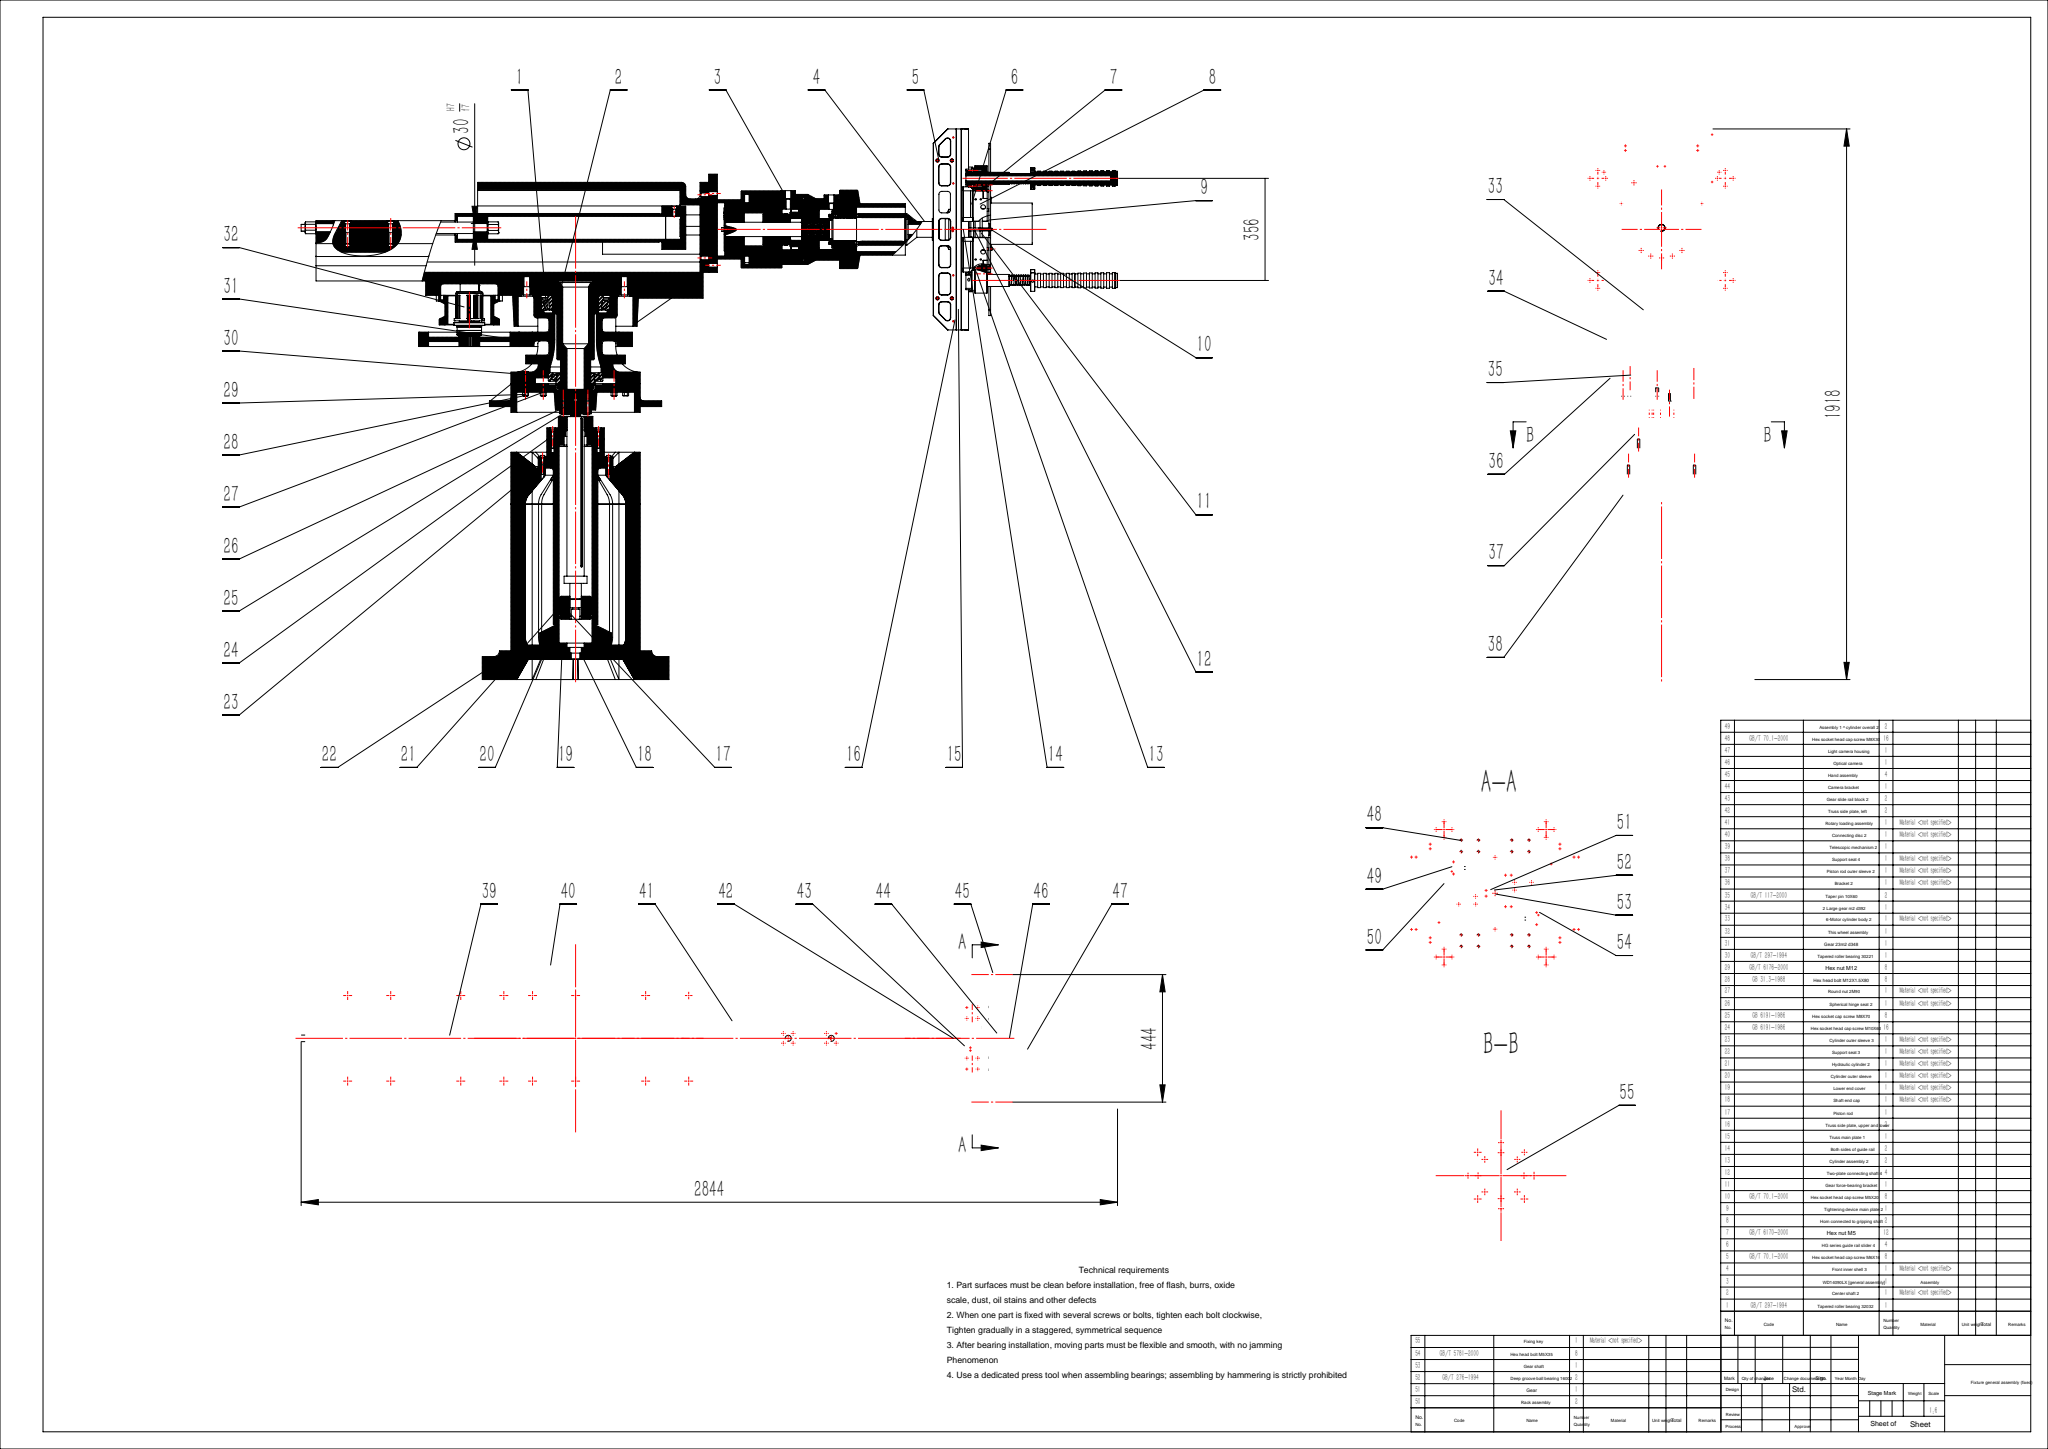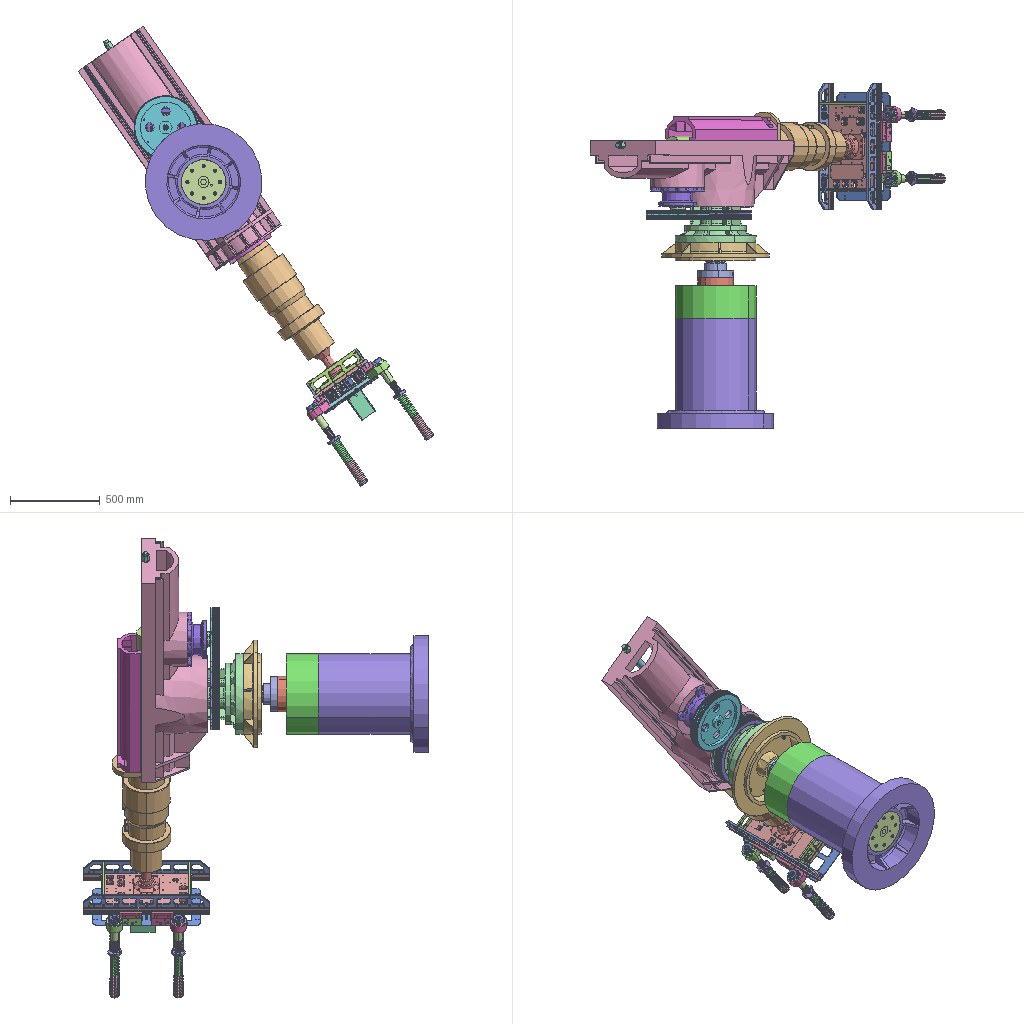Assembly | SolidWorks | 123 different items | 407 placed | box 1975 x 1918 x 2559 mm
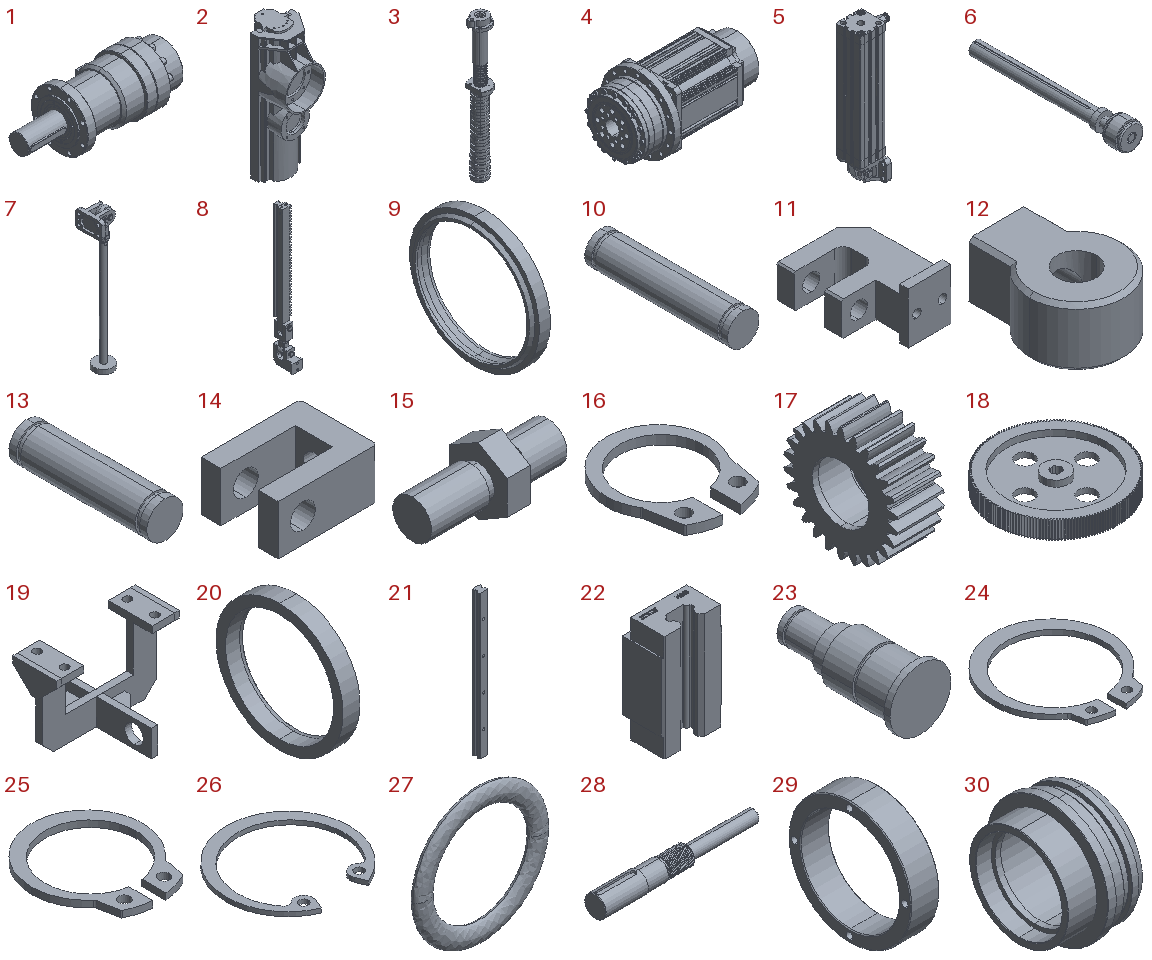Parts list (item | name | quantity | parent item | size | volume | features):
1 | (subassembly) | x1 | - | - | 15807890 mm3 | features InContextFeatHolder 12, ReferencePattern 9, CompositeCurve 5, HoleSeries 3, AEMSimFeature 1, Cut 1, LocalCirPattern 1
2 | (subassembly) | x1 | - | 440 x 501.037 x 1420 mm | 76024148 mm3 | -
3 | (subassembly) | x4 | - | 78.987 x 76 x 528 mm | 773496 mm3 | features CompositeCurve 5
4 | (subassembly) | x1 | - | 182 x 107 x 107 mm | 904156 mm3 | -
5 | (subassembly) | x2 | - | 74.5 x 58 x 297.75 mm | 433626 mm3 | -
6 | (subassembly) | x1 | - | 115 x 705.59 x 115 mm | 2459406 mm3 | -
7 | (subassembly) | x2 | - | 52 x 56 x 300.673 mm | 74670 mm3 | features CompositeCurve 1
8 | (subassembly) | x2 | - | 30 x 59.858 x 379 mm | 198364 mm3 | -
9 | - | x2 | in 1 | 6.5 x 58 x 58 mm | 3242 mm3 | features Revolution 2
10 | - | x2 | in 8 | 10 x 45 x 10 mm | 3498 mm3 | features Revolution 1
11 | - | x2 | in 8 | 45 x 57 x 30 mm | 31506 mm3 | features ICE 4, HoleWzd 3, Chamfer 2, Extrusion 1, Fillet 1
12 | - | x2 | in 8 | 24 x 32 x 15 mm | 6636 mm3 | features HoleWzd 2, Chamfer 1, Extrusion 1
13 | - | x2 | in 8 | 10 x 38 x 10 mm | 2949 mm3 | features Revolution 1
14 | - | x2 | in 8 | 40 x 31 x 20 mm | 13956 mm3 | features HoleWzd 3, Chamfer 1, Extrusion 1, ICE 1
15 | - | x2 | in 8 | 35 x 15 x 17.321 mm | 3350 mm3 | features Revolution 2, Extrusion 1
16 | - | x4 | in 8 | 11.5 x 13.997 x 1 mm | 50.603 mm3 | features Extrusion 1
17 | - | x1 | - | 23 x 55.72 x 56 mm | 29460 mm3 | features ICE 26, RevCut 1, Revolution 1
18 | - | x1 | - | 351.968 x 352 x 50 mm | 2206869 mm3 | features ICE 5, CirPattern 1, MirrorPattern 1, RefAxis 1, RevCut 1, Revolution 1
19 | - | x1 | - | 111 x 106 x 71 mm | 53566 mm3 | features BaseBody 7
20 | - | x4 | in 1 | 8 x 60 x 60 mm | 5343 mm3 | features Revolution 2
21 | - | x2 | in 8 | 15 x 15 x 270 mm | 50125 mm3 | features Draft 2, Fillet 2, ICE 2, Chamfer 1, Extrusion 1, HoleWzd 1
22 | - | x2 | - | 34 x 23.7 x 61.7 mm | 37116 mm3 | features Chamfer 35, ICE 15, Draft 12, Fillet 3, Extrusion 1, HoleWzd 1
23 | - | x1 | - | 30 x 63 x 30 mm | 23893 mm3 | features Revolution 1
24 | - | x1 | - | 28.2 x 30.881 x 1.2 mm | 270.422 mm3 | features Extrusion 1
25 | - | x1 | - | 16.8 x 19.352 x 1 mm | 87.473 mm3 | features Extrusion 1
26 | - | x1 | - | 34.4 x 33.091 x 1.2 mm | 290.13 mm3 | features Extrusion 1
27 | - | x2 | in 1 | 29.8 x 2.4 x 29.8 mm | 636.708 mm3 | features Revolution 2
28 | - | x1 | in 1 | 630 x 85 x 85 mm | 2283899 mm3 | features ICE 6, Chamfer 4, Fillet 2, CirPattern 1, Extrusion 1, Helix 1, HoleWzd 1, MirrorPattern 1, SweepCut 1
29 | - | x1 | in 1 | 35 x 150 x 150 mm | 215991 mm3 | features Chamfer 1, Extrusion 1, HoleWzd 1
30 | - | x1 | in 1 | 86 x 147 x 147 mm | 431094 mm3 | features ICE 5, Chamfer 3, Cavity 1, Extrusion 1
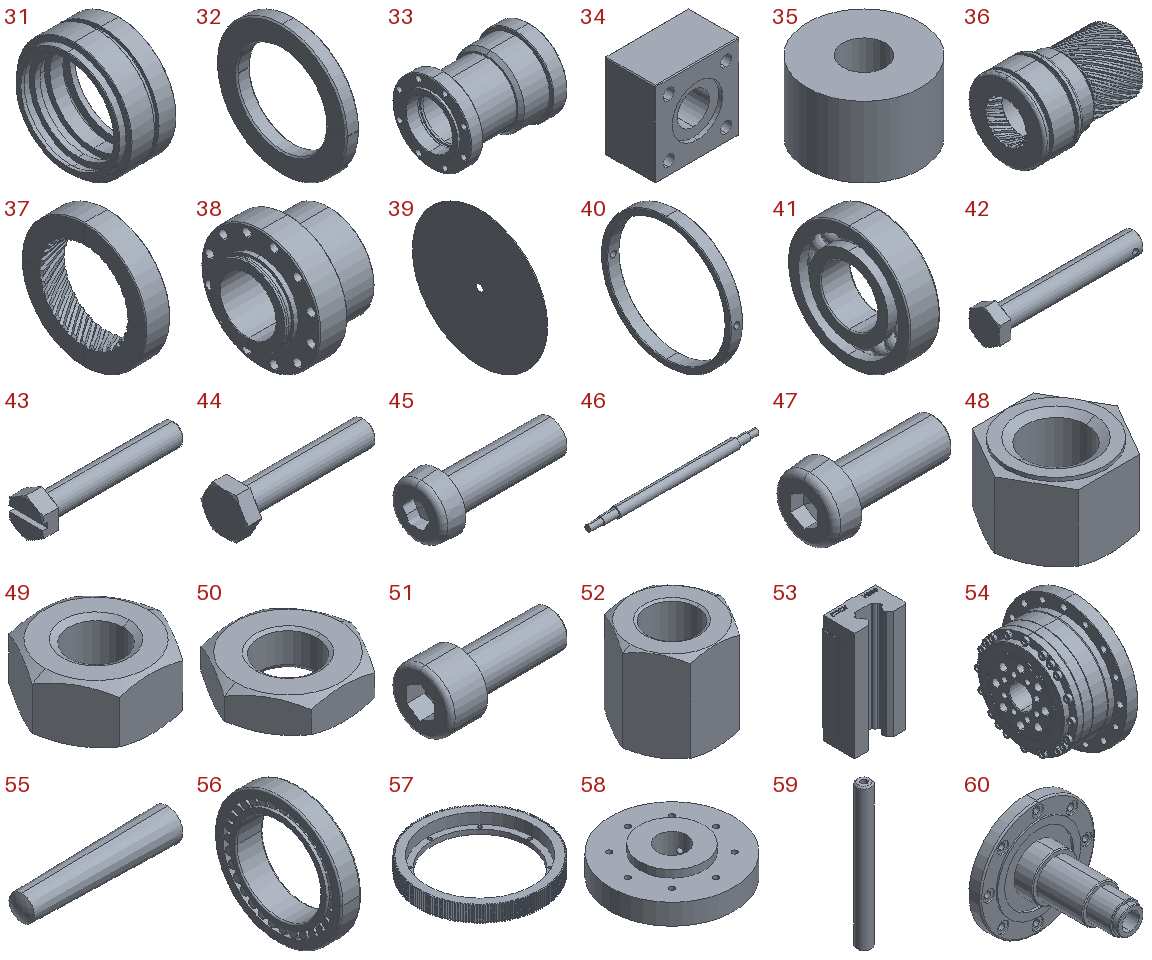31 | - | x1 | in 1 | 47 x 105 x 105 mm | 121428 mm3 | features Cavity 1, Chamfer 1, Extrusion 1, ICE 1
32 | - | x1 | in 1 | 10 x 94.999 x 95 mm | 37048 mm3 | features Chamfer 1, Extrusion 1, ICE 1
33 | - | x1 | in 1 | 317 x 249 x 249 mm | 6036986 mm3 | features Chamfer 8, HoleWzd 6, ICE 5, Cut 1, Fillet 1, LibraryFeature 1, Revolution 1
34 | - | x2 | in 1 | 50 x 30 x 50 mm | 59677 mm3 | features HoleWzd 2, Chamfer 1, Extrusion 1, ICE 1
35 | - | x1 | in 2 | 80 x 80 x 50 mm | 215984 mm3 | features Extrusion 1
36 | - | x1 | in 1 | 196 x 140 x 140 mm | 1596152 mm3 | features ICE 6, Cavity 2, Chamfer 2, CirPattern 2, Fillet 2, Helix 2, SweepCut 2, Extrusion 1
37 | - | x1 | in 1 | 30 x 155 x 155 mm | 292361 mm3 | features Chamfer 2, CirPattern 2, Extrusion 1, Helix 1, ICE 1, SweepCut 1
38 | - | x1 | in 1 | 168.5 x 244 x 244 mm | 4079273 mm3 | features ICE 6, Chamfer 3, Cavity 2, Extrusion 1, HoleWzd 1
39 | - | x1 | in 1 | 1 x 150 x 150 mm | 17590 mm3 | features ICE 5, CirPattern 3, Extrusion 1
40 | - | x1 | in 1 | 10 x 105 x 105 mm | 15354 mm3 | features Chamfer 1, Extrusion 1, HoleWzd 1
41 | - | x2 | - | 8 x 32 x 32 mm | 3760 mm3 | features Revolution 3, CirPattern 1, Fillet 1
42 | - | x8 | - | 87.32 x 17.73 x 20.473 mm | 10914 mm3 | features RevCut 3, Boss 1, Chamfer 1, Cut 1, Extrusion 1, Fillet 1, LPattern 1
43 | - | x4 | - | 34.15 x 7.78 x 8.984 mm | 788.587 mm3 | features RevCut 2, Boss 1, Chamfer 1, Cut 1, Extrusion 1, Fillet 1, LPattern 1, Revolution 1
44 | - | x8 | - | 34 x 11.547 x 10 mm | 1183 mm3 | features RevCut 3, Boss 1, Chamfer 1, Extrusion 1, Fillet 1, LPattern 1
45 | - | x12 | - | 23.9 x 10 x 10 mm | 812.082 mm3 | features BlendCut 1, Cut 1, Extrusion 1, Fillet 1, LPattern 1, RevCut 1, Revolution 1
46 | - | x1 | in 2 | 685 x 40 x 40 mm | 729842 mm3 | features Revolution 1
47 | - | x98 | in 2, 5 | 19.9 x 10 x 10 mm | 696.754 mm3 | features Cut 2, Fillet 2, Boss 1, Chamfer 1, Extrusion 1, LPattern 1, RevCut 1
48 | - | x8 | - | 20.785 x 18 x 12.6 mm | 2391 mm3 | features RevCut 4, Chamfer 2, Boss 1, Extrusion 1, LPattern 1
49 | - | x12 | - | 11.547 x 10 x 5.2 mm | 340.667 mm3 | features RevCut 2, Chamfer 1, Extrusion 1, LPattern 1
50 | - | x2 | in 7 | 18.475 x 16 x 5 mm | 807.232 mm3 | features RevCut 2, Chamfer 1, Extrusion 1, LPattern 1
51 | - | x44 | in 8 | 28 x 13 x 13 mm | 1916 mm3 | features Fillet 2, RevCut 2, Boss 1, Chamfer 1, Cut 1, Extrusion 1, LPattern 1
52 | - | x2 | in 2 | 41.569 x 36 x 38 mm | 29600 mm3 | features RevCut 2, Chamfer 1, Extrusion 1, LPattern 1
53 | - | x4 | - | 60 x 36 x 120.7 mm | 197221 mm3 | features Draft 43, Chamfer 42, ICE 29, Fillet 8, BaseBody 1, HoleWzd 1
54 | - | x1 | in 4 | 50 x 107 x 107 mm | 232615 mm3 | features ICE 1, MBimport 1
55 | - | x2 | - | 60 x 12.304 x 12.304 mm | 5767 mm3 | features Revolution 1
56 | - | x2 | - | 51 x 240 x 240 mm | 870409 mm3 | features Revolution 3, CirPattern 1
57 | - | x1 | - | 395.972 x 395.972 x 50 mm | 1324995 mm3 | features ICE 3, CirPattern 1, RefAxis 1, RevCut 1, Revolution 1
58 | - | x1 | - | 250 x 250 x 57.13 mm | 2053671 mm3 | features ICE 4, Extrusion 1, RevCut 1
59 | - | x4 | - | 10 x 10 x 100 mm | 7469 mm3 | features Revolution 1
60 | - | x1 | - | 400 x 377 x 400 mm | 7916207 mm3 | features ICE 5, Chamfer 2, Revolution 1
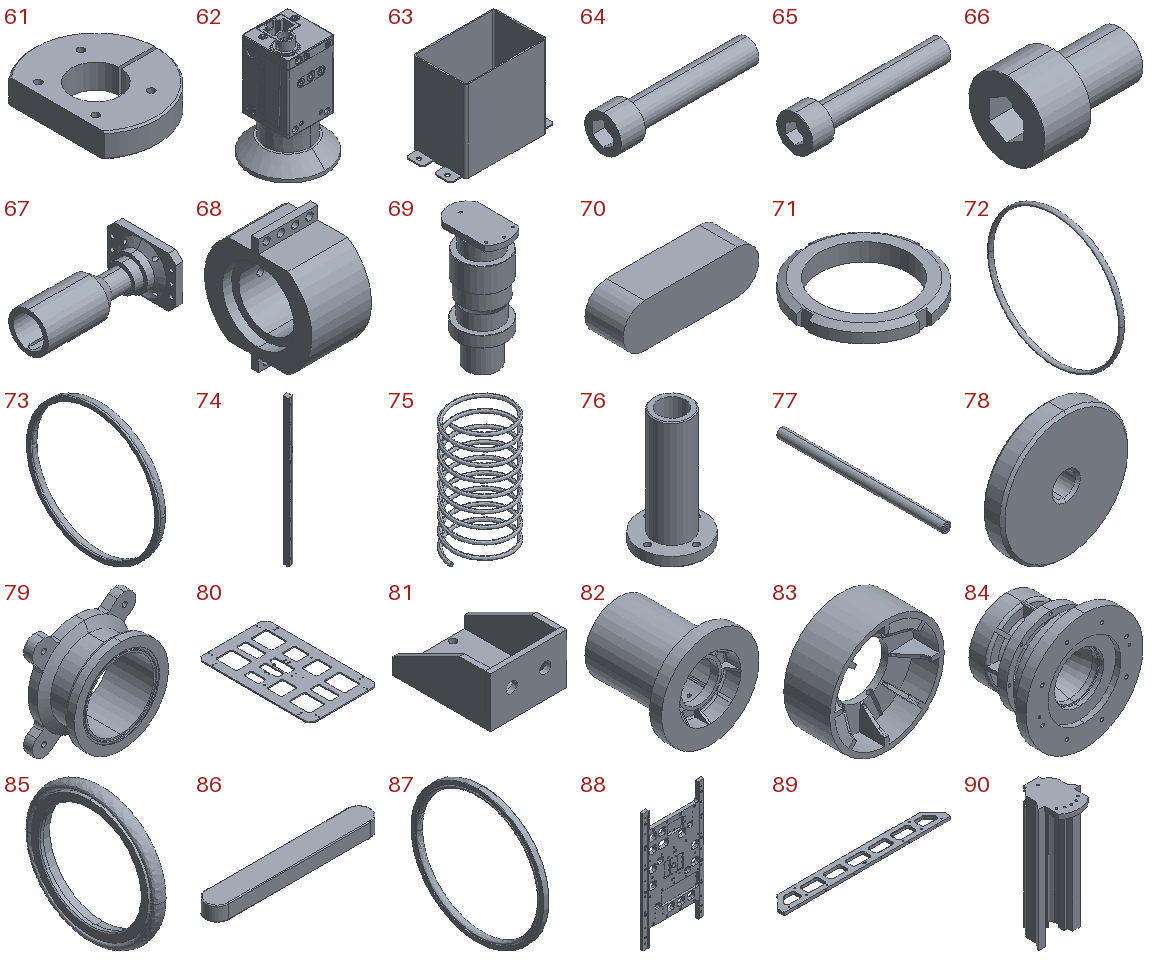61 | - | x4 | in 3 | 61.987 x 76 x 15 mm | 44061 mm3 | features HoleWzd 3, Chamfer 1, Extrusion 1, ICE 1, RevCut 1
62 | - | x1 | - | 46.38 x 46.38 x 70.1 mm | 45719 mm3 | features BaseBody 15
63 | - | x1 | - | 184 x 94 x 145 mm | 138135 mm3 | features BaseBody 5
64 | - | x10 | in 1 | 96 x 24 x 24 mm | 21953 mm3 | features BlendCut 1, Cut 1, Fillet 1, RevCut 1, Revolution 1
65 | - | x8 | in 1 | 41 x 10 x 10 mm | 1393 mm3 | features BlendCut 1, Cut 1, Fillet 1, RevCut 1, Revolution 1
66 | - | x1 | in 1 | 20 x 13 x 13 mm | 1535 mm3 | features BlendCut 1, Cut 1, Fillet 1, RevCut 1, Revolution 1
67 | - | x1 | - | 346 x 190 x 140 mm | 1651422 mm3 | features ICE 6, Revolution 2, RefAxis 1
68 | - | x1 | in 2 | 83 x 150 x 161 mm | 1012168 mm3 | features ICE 5, Revolution 1
69 | - | x1 | - | 273 x 341.706 x 685 mm | 8218531 mm3 | features ICE 4, Chamfer 2, Extrusion 1, RefAxis 1, Revolution 1
70 | - | x1 | - | 25 x 7 x 8 mm | 1304 mm3 | features Extrusion 1
71 | - | x1 | - | 124.423 x 124.423 x 18 mm | 93238 mm3 | features Extrusion 1, ICE 1, RevCut 1
72 | - | x1 | in 1 | 4 x 105 x 105 mm | 2430 mm3 | features Revolution 2
73 | - | x2 | in 1 | 9.6 x 155 x 155 mm | 16985 mm3 | features Revolution 3
74 | - | x2 | - | 28 x 26 x 700 mm | 404636 mm3 | features ICE 8, Draft 4, Fillet 2, Chamfer 1, Extrusion 1, HoleWzd 1
75 | - | x4 | in 3 | 36 x 36 x 74 mm | 3015 mm3 | features BaseBody 1
76 | - | x4 | in 3 | 72 x 72 x 131 mm | 113425 mm3 | features HoleWzd 2, Revolution 2, Chamfer 1, ICE 1
77 | - | x4 | in 3 | 30 x 520 x 30 mm | 241731 mm3 | features BaseBody 2
78 | - | x4 | in 3 | 50 x 8 x 50 mm | 15014 mm3 | features Revolution 1
79 | - | x1 | - | 230.312 x 103 x 230.312 mm | 1234015 mm3 | features ICE 5, CirPattern 2, Revolution 1
80 | - | x1 | - | 360 x 600 x 6 mm | 820919 mm3 | features Extrusion 1
81 | - | x1 | - | 46 x 58 x 30 mm | 17928 mm3 | features BaseBody 4
82 | - | x1 | - | 650 x 611.2 x 650 mm | 36285371 mm3 | features ICE 4, Revolution 2, CirPattern 1
83 | - | x1 | - | 450 x 180.45 x 450 mm | 8519490 mm3 | features ICE 3, Revolution 2, CirPattern 1
84 | - | x1 | - | 450 x 299 x 450 mm | 13734208 mm3 | features ICE 5, MirrorPattern 2, RevCut 2, Revolution 2, CirPattern 1
85 | - | x2 | in 1 | 6.3 x 65.5 x 65.5 mm | 7151 mm3 | features Revolution 3
86 | - | x2 | in 1 | 157 x 22 x 14 mm | 46809 mm3 | features Extrusion 1, Fillet 1
87 | - | x2 | in 1 | 6.3 x 140 x 140 mm | 18044 mm3 | features Revolution 3
88 | - | x1 | - | 360 x 20 x 700 mm | 2898584 mm3 | features ICE 24, HoleWzd 12, RevCut 4, Fillet 2, Chamfer 1, Extrusion 1
89 | - | x2 | - | 700 x 80 x 12 mm | 406374 mm3 | features ICE 7, HoleWzd 4, Chamfer 1, Extrusion 1, Fillet 1
90 | - | x1 | in 2 | 275.23 x 313.202 x 805 mm | 12308748 mm3 | features ICE 9, Fillet 2, Extrusion 1
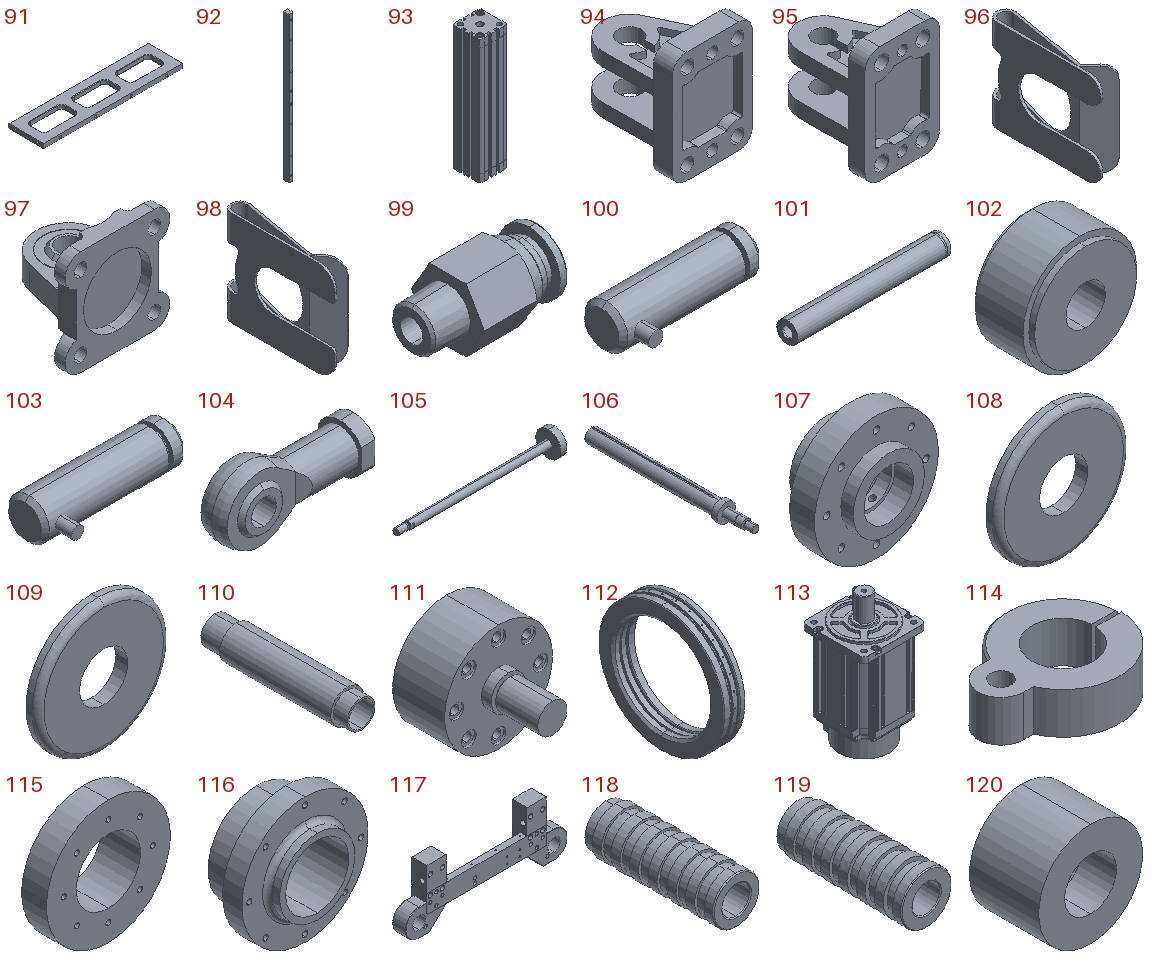91 | - | x2 | - | 318 x 80 x 10 mm | 157548 mm3 | features HoleWzd 3, ICE 3, Chamfer 1, Extrusion 1, Fillet 1
92 | - | x2 | in 2 | 64 x 50 x 1288 mm | 2493147 mm3 | features ICE 3, Extrusion 1, MirrorPattern 1
93 | - | x2 | in 5 | - | - | features ICE 104, RefSurface 48, Draft 32, HoleWzd 7, Fillet 3, Chamfer 2, Extrusion 1
94 | - | x2 | in 5 | 41.75 x 50 x 58 mm | 28986 mm3 | features ICE 9, Fillet 2, HoleWzd 2, RevCut 2, Draft 1, Extrusion 1
95 | - | x2 | in 7 | 36 x 44 x 56 mm | 21149 mm3 | features ICE 10, Fillet 2, HoleWzd 2, RevCut 2, Extrusion 1
96 | - | x2 | in 7 | 4.9 x 22 x 18 mm | 263.312 mm3 | features Fillet 2, BaseBody 1, ICE 1
97 | - | x2 | in 5 | 54 x 42 x 54 mm | 25810 mm3 | features ICE 8, Fillet 3, HoleWzd 3, BaseBody 1
98 | - | x2 | in 5 | 5 x 25.9 x 22 mm | 386.551 mm3 | features Fillet 3, ICE 2, BaseBody 1
99 | - | x4 | in 5 | 28 x 16.166 x 14 mm | 2490 mm3 | features Fillet 2, BaseBody 1, Chamfer 1, HoleWzd 1, ICE 1, Revolution 1
100 | - | x2 | in 5 | 39 x 16 x 12 mm | 4350 mm3 | features Revolution 2, Chamfer 1
101 | - | x1 | in 2 | 733.26 x 100 x 100 mm | 2092822 mm3 | features ICE 2, Revolution 1
102 | - | x1 | in 6 | 115 x 60 x 115 mm | 523160 mm3 | features Revolution 1
103 | - | x2 | in 7 | 35 x 14 x 10 mm | 2719 mm3 | features Revolution 2, Chamfer 1
104 | - | x2 | in 7 | 57 x 17 x 28 mm | 10383 mm3 | features Draft 2, HoleWzd 2, ICE 2, BaseBody 1, Chamfer 1
105 | - | x2 | in 7 | 253.7 x 40 x 40 mm | 39349 mm3 | features ICE 6, Draft 2, Chamfer 1, Fillet 1, Revolution 1
106 | - | x1 | in 6 | 80 x 705.59 x 80 mm | 1778352 mm3 | features ICE 3, Revolution 1
107 | - | x1 | - | 200 x 100 x 200 mm | 1489766 mm3 | features ICE 4, RevCut 1, Revolution 1
108 | - | x1 | in 6 | 109 x 10 x 109 mm | 78947 mm3 | features Revolution 1
109 | - | x1 | in 6 | 109 x 10 x 109 mm | 78947 mm3 | features Revolution 1
110 | - | x1 | - | 155 x 684.63 x 155 mm | 4883903 mm3 | features Revolution 1
111 | - | x1 | - | 110 x 108 x 110 mm | 515028 mm3 | features ICE 6, Revolution 1
112 | - | x2 | in 1 | 19 x 105 x 105 mm | 55115 mm3 | features BaseBody 4
113 | - | x1 | in 4 | 80 x 90 x 164 mm | 671541 mm3 | features MBimport 1
114 | - | x4 | in 3 | 68.482 x 55 x 20 mm | 34812 mm3 | features HoleWzd 3, Chamfer 1, Extrusion 1, ICE 1, RevCut 1
115 | - | x1 | - | 250 x 80 x 250 mm | 2252522 mm3 | features ICE 1, Revolution 1
116 | - | x1 | - | 260 x 125 x 260 mm | 2840283 mm3 | features ICE 3, Revolution 1
117 | - | x2 | - | 532 x 49 x 194 mm | 1579293 mm3 | features BaseBody 3, HoleWzd 2, ICE 2
118 | - | x4 | in 3 | 50 x 140 x 50 mm | 149689 mm3 | features Revolution 1
119 | - | x4 | in 3 | 54.97 x 140 x 54.97 mm | 171748 mm3 | features Revolution 1
120 | - | x1 | - | 60 x 40 x 60 mm | 73933 mm3 | features Revolution 1
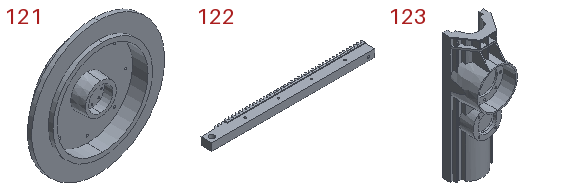121 | - | x1 | - | 600 x 100 x 600 mm | 9551199 mm3 | features ICE 10, RefAxis 2, CirPattern 1, MirrorPattern 1, RevCut 1, Revolution 1, Rib 1
122 | - | x2 | in 8 | 295 x 24 x 15 mm | 85099 mm3 | features ICE 46, Draft 42, HoleWzd 5, Extrusion 1
123 | - | x1 | in 2 | 440 x 367.835 x 1348 mm | 54378577 mm3 | features ICE 24, Fillet 8, MirrorPattern 4, CirPattern 2, Extrusion 1
Mates (type | each side: item.copy, entity, surface, feature), first 275 of 722 lines:
In the top assembly
Concentric | 88.1 face cylinder M6 六角头Bolt的柱形沉头Hole 2 | 89.1 face cylinder Ø5.0 (5) DiameterHole 2
Coincident | 88.1 face plane Boss-Extrude 1 | 89.1 face plane Boss-Extrude 1 | 2 times
Concentric | 88.1 face cylinder M6 六角头Bolt的柱形沉头Hole 2 | 45.1 face cone BaseHead
Coincident | 88.1 face plane M6 六角头Bolt的柱形沉头Hole 2 | 45.1 face plane BaseHead
Concentric | 88.1 face cylinder M6 六角头Bolt的柱形沉头Hole 2 | 45.2 face cone BaseHead
Coincident | 88.1 face plane M6 六角头Bolt的柱形沉头Hole 2 | 45.2 face plane BaseHead
Concentric | 88.1 face cylinder M6 六角头Bolt的柱形沉头Hole 2 | 45.3 face cone BaseHead
Coincident | 88.1 face plane M6 六角头Bolt的柱形沉头Hole 2 | 45.3 face plane BaseHead
Concentric | 88.1 face cylinder M6 六角头Bolt的柱形沉头Hole 2 | 45.4 face cone BaseHead
Coincident | 88.1 face plane M6 六角头Bolt的柱形沉头Hole 2 | 45.4 face plane BaseHead
Concentric | 88.1 face cylinder M6 六角头Bolt的柱形沉头Hole 2 | 45.5 face cone BaseHead
Coincident | 88.1 face plane M6 六角头Bolt的柱形沉头Hole 2 | 45.5 face plane BaseHead
Concentric | 88.1 face cylinder M6 六角头Bolt的柱形沉头Hole 2 | 45.6 face cone BaseHead
Coincident | 88.1 face plane M6 六角头Bolt的柱形沉头Hole 2 | 45.6 face plane BaseHead
Concentric | 88.1 face cylinder M6 六角头Bolt的柱形沉头Hole 2 | 45.7 face cone BaseHead
Coincident | 88.1 face plane M6 六角头Bolt的柱形沉头Hole 2 | 45.7 face plane BaseHead
Concentric | 88.1 face cylinder M6 六角头Bolt的柱形沉头Hole 2 | 89.2 face cylinder Ø5.0 (5) DiameterHole 2 | 2 times
Coincident | 88.1 face plane Boss-Extrude 1 | 89.2 face plane Boss-Extrude 1
Concentric | 88.1 face cylinder M6 六角头Bolt的柱形沉头Hole 1 | 91.1 face cylinder Ø5.0 (5) DiameterHole 3 | 2 times
Coincident | 88.1 face plane Boss-Extrude 1 | 91.1 face plane Boss-Extrude 1
Concentric | 88.1 face cylinder M6 六角头Bolt的柱形沉头Hole 1 | 91.2 face cylinder Ø5.0 (5) DiameterHole 3 | 2 times
Coincident | 88.1 face plane Boss-Extrude 1 | 91.2 face plane Boss-Extrude 1
Concentric | 88.1 face cylinder M6 六角头Bolt的柱形沉头Hole 1 | 47.1 face cylinder BaseBody
Coincident | 88.1 face plane M6 六角头Bolt的柱形沉头Hole 1 | 47.1 face plane BaseHead
Concentric | 88.1 face cylinder M6 六角头Bolt的柱形沉头Hole 1 | 47.2 face cylinder BaseBody
Coincident | 88.1 face plane M6 六角头Bolt的柱形沉头Hole 1 | 47.2 face plane BaseHead
Concentric | 88.1 face cylinder M6 六角头Bolt的柱形沉头Hole 1 | 47.3 face cylinder BaseBody
Coincident | 88.1 face plane M6 六角头Bolt的柱形沉头Hole 1 | 47.3 face plane BaseHead
Concentric | 88.1 face cylinder M6 六角头Bolt的柱形沉头Hole 1 | 47.4 face cylinder BaseBody
Coincident | 88.1 face plane M6 六角头Bolt的柱形沉头Hole 1 | 47.4 face plane BaseHead
Concentric | 88.1 face cylinder M6 六角头Bolt的柱形沉头Hole 1 | 47.5 face cylinder BaseBody
Coincident | 88.1 face plane M6 六角头Bolt的柱形沉头Hole 1 | 47.5 face plane BaseHead
Concentric | 88.1 face cylinder M6 六角头Bolt的柱形沉头Hole 1 | 47.6 face cylinder BaseBody
Coincident | 88.1 face plane M6 六角头Bolt的柱形沉头Hole 1 | 47.6 face plane BaseHead
Concentric | 88.1 face cylinder M6 六角头Bolt的柱形沉头Hole 1 | 47.7 face cylinder BaseBody
Coincident | 88.1 face plane M6 六角头Bolt的柱形沉头Hole 1 | 47.7 face plane BaseHead
Concentric | 88.1 face cylinder M6 六角头Bolt的柱形沉头Hole 1 | 47.8 face cylinder BaseBody
Coincident | 88.1 face plane M6 六角头Bolt的柱形沉头Hole 1 | 47.8 face plane BaseHead
Concentric | 89.2 face cylinder M6 六角头Bolt的柱形沉头Hole 1 | 47.9 face cylinder BaseBody
Coincident | 89.2 face plane M6 六角头Bolt的柱形沉头Hole 1 | 47.9 face plane BaseHead
Concentric | 89.2 face cylinder M6 六角头Bolt的柱形沉头Hole 1 | 47.10 face cylinder BaseBody
Coincident | 89.2 face plane M6 六角头Bolt的柱形沉头Hole 1 | 47.10 face plane BaseHead
Concentric | 89.1 face cylinder M6 六角头Bolt的柱形沉头Hole 1 | 47.11 face cylinder BaseBody
Coincident | 89.1 face plane M6 六角头Bolt的柱形沉头Hole 1 | 47.11 face plane BaseHead
Concentric | 89.1 face cylinder M6 六角头Bolt的柱形沉头Hole 1 | 47.12 face cylinder BaseBody
Coincident | 89.1 face plane M6 六角头Bolt的柱形沉头Hole 1 | 47.12 face plane BaseHead
Concentric | 89.1 face cylinder M6 六角头Bolt的柱形沉头Hole 1 | 47.13 face cylinder BaseBody
Coincident | 89.1 face plane M6 六角头Bolt的柱形沉头Hole 1 | 47.13 face plane BaseHead
Concentric | 89.1 face cylinder M6 六角头Bolt的柱形沉头Hole 1 | 47.14 face cylinder BaseBody
Concentric | 89.2 face cylinder M6 六角头Bolt的柱形沉头Hole 1 | 47.15 face cylinder BaseBody
Coincident | 89.2 face plane M6 六角头Bolt的柱形沉头Hole 1 | 47.15 face plane BaseHead
Concentric | 89.2 face cylinder M6 六角头Bolt的柱形沉头Hole 1 | 47.16 face cylinder BaseBody
Coincident | 89.2 face plane M6 六角头Bolt的柱形沉头Hole 1 | 47.16 face plane BaseHead
Coincident | 89.1 face plane M6 六角头Bolt的柱形沉头Hole 1 | 47.14 face plane BaseHead
Coincident | 88.1 face plane Cut-Extrude 3 | 74.1 face plane Boss-Extrude 1
Coincident | 88.1 face plane Boss-Extrude 1 | 74.1 face plane Boss-Extrude 1
Concentric | 88.1 face cylinder Ø6.8 (6.8) DiameterHole 1 | 74.1 face cylinder M8 六角头Bolt的柱形沉头Hole 1
Coincident | 88.1 face plane Cut-Extrude 2 | 74.2 face plane Boss-Extrude 1
Coincident | 88.1 face plane Boss-Extrude 1 | 74.2 face plane Boss-Extrude 1
Concentric | 88.1 face cylinder Ø6.8 (6.8) DiameterHole 1 | 74.2 face cylinder M8 六角头Bolt的柱形沉头Hole 1
Concentric | 74.2 face cylinder M8 六角头Bolt的柱形沉头Hole 1 | 47.17 face cylinder BaseBody
Coincident | 74.2 face plane M8 六角头Bolt的柱形沉头Hole 1 | 47.17 face plane BaseHead
Concentric | 74.1 face cylinder M8 六角头Bolt的柱形沉头Hole 1 | 47.18 face cylinder BaseBody
Coincident | 74.1 face plane M8 六角头Bolt的柱形沉头Hole 1 | 47.18 face plane BaseHead
Concentric | 74.1 face cylinder M8 六角头Bolt的柱形沉头Hole 1 | 47.19 face cylinder BaseBody
Coincident | 74.1 face plane M8 六角头Bolt的柱形沉头Hole 1 | 47.19 face plane BaseHead
Concentric | 74.1 face cylinder M8 六角头Bolt的柱形沉头Hole 1 | 47.20 face cylinder BaseBody
Coincident | 74.1 face plane M8 六角头Bolt的柱形沉头Hole 1 | 47.20 face plane BaseHead
Concentric | 74.1 face cylinder M8 六角头Bolt的柱形沉头Hole 1 | 47.21 face cylinder BaseBody
Coincident | 74.1 face plane M8 六角头Bolt的柱形沉头Hole 1 | 47.21 face plane BaseHead
Concentric | 74.1 face cylinder M8 六角头Bolt的柱形沉头Hole 1 | 47.22 face cylinder BaseBody
Coincident | 74.1 face plane M8 六角头Bolt的柱形沉头Hole 1 | 47.22 face plane BaseHead
Concentric | 74.1 face cylinder M8 六角头Bolt的柱形沉头Hole 1 | 47.23 face cylinder BaseBody
Coincident | 74.1 face plane M8 六角头Bolt的柱形沉头Hole 1 | 47.23 face plane BaseHead
Concentric | 74.1 face cylinder M8 六角头Bolt的柱形沉头Hole 1 | 47.24 face cylinder BaseBody
Coincident | 74.1 face plane M8 六角头Bolt的柱形沉头Hole 1 | 47.24 face plane BaseHead
Concentric | 74.1 face cylinder M8 六角头Bolt的柱形沉头Hole 1 | 47.25 face cylinder BaseBody
Coincident | 74.1 face plane M8 六角头Bolt的柱形沉头Hole 1 | 47.25 face plane BaseHead
Concentric | 74.1 face cylinder M8 六角头Bolt的柱形沉头Hole 1 | 47.26 face cylinder BaseBody
Coincident | 74.1 face plane M8 六角头Bolt的柱形沉头Hole 1 | 47.26 face plane BaseHead
Concentric | 74.2 face cylinder M8 六角头Bolt的柱形沉头Hole 1 | 47.27 face cylinder BaseBody
Coincident | 74.2 face plane M8 六角头Bolt的柱形沉头Hole 1 | 47.27 face plane BaseHead
Concentric | 74.2 face cylinder M8 六角头Bolt的柱形沉头Hole 1 | 47.28 face cylinder BaseBody
Coincident | 74.2 face plane M8 六角头Bolt的柱形沉头Hole 1 | 47.28 face plane BaseHead
Concentric | 74.2 face cylinder M8 六角头Bolt的柱形沉头Hole 1 | 47.29 face cylinder BaseBody
Coincident | 74.2 face plane M8 六角头Bolt的柱形沉头Hole 1 | 47.29 face plane BaseHead
Concentric | 74.2 face cylinder M8 六角头Bolt的柱形沉头Hole 1 | 47.30 face cylinder BaseBody
Coincident | 74.2 face plane M8 六角头Bolt的柱形沉头Hole 1 | 47.30 face plane BaseHead
Concentric | 74.2 face cylinder M8 六角头Bolt的柱形沉头Hole 1 | 47.31 face cylinder BaseBody
Coincident | 74.2 face plane M8 六角头Bolt的柱形沉头Hole 1 | 47.31 face plane BaseHead
Concentric | 74.2 face cylinder M8 六角头Bolt的柱形沉头Hole 1 | 47.32 face cylinder BaseBody
Coincident | 74.2 face plane M8 六角头Bolt的柱形沉头Hole 1 | 47.32 face plane BaseHead
Concentric | 74.2 face cylinder M8 六角头Bolt的柱形沉头Hole 1 | 47.33 face cylinder BaseBody
Coincident | 74.2 face plane M8 六角头Bolt的柱形沉头Hole 1 | 47.33 face plane BaseHead
Concentric | 74.2 face cylinder M8 六角头Bolt的柱形沉头Hole 1 | 47.34 face cylinder BaseBody
Coincident | 74.2 face plane M8 六角头Bolt的柱形沉头Hole 1 | 47.34 face plane BaseHead
Coincident | 74.2 face plane Boss-Extrude 1 | 53.1 face plane Cut-Extrude 8 | 2 times
Coincident | 74.2 face plane Boss-Extrude 1 | 53.2 face plane Cut-Extrude 8 | 2 times
Coincident | 74.1 face plane Boss-Extrude 1 | 53.3 face plane Cut-Extrude 8 | 2 times
Coincident | 74.1 face plane Boss-Extrude 1 | 53.4 face plane Cut-Extrude 8 | 2 times
Coincident | 53.2 face plane Boss-Extrude 10 | 53.4 face plane Boss-Extrude 10
Coincident | 53.1 face plane Boss-Extrude 10 | 53.3 face plane Boss-Extrude 10
Coincident | 88.1 face plane Cut-Extrude 22 | 22.1 face plane Boss-Extrude 1
Concentric | 88.1 face cylinder M4 六角头机械Screw的柱形沉头Hole 1 | 22.1 face cylinder Ø4.0 (4) DiameterHole 1 | 2 times
Coincident | 88.1 face plane Cut-Extrude 21 | 22.2 face plane Boss-Extrude 1
Concentric | 88.1 face cylinder M4 六角头机械Screw的柱形沉头Hole 1 | 22.2 face cylinder Ø4.0 (4) DiameterHole 1 | 2 times
Concentric | 88.1 face cylinder M4 六角头机械Screw的柱形沉头Hole 1 | 51.1 face cylinder BaseBody
Coincident | 88.1 face plane M4 六角头机械Screw的柱形沉头Hole 1 | 51.1 face plane BaseHead
Concentric | 88.1 face cylinder M4 六角头机械Screw的柱形沉头Hole 1 | 51.2 face cylinder BaseBody
Coincident | 88.1 face plane M4 六角头机械Screw的柱形沉头Hole 1 | 51.2 face plane BaseHead
Concentric | 88.1 face cylinder M4 六角头机械Screw的柱形沉头Hole 1 | 51.3 face cylinder BaseBody
Coincident | 88.1 face plane M4 六角头机械Screw的柱形沉头Hole 1 | 51.3 face plane BaseHead
Concentric | 88.1 face cylinder M4 六角头机械Screw的柱形沉头Hole 1 | 51.4 face cylinder BaseBody
Coincident | 88.1 face plane M4 六角头机械Screw的柱形沉头Hole 1 | 51.4 face plane BaseHead
Concentric | 88.1 face cylinder M4 六角头机械Screw的柱形沉头Hole 1 | 51.5 face cylinder BaseBody
Coincident | 88.1 face plane M4 六角头机械Screw的柱形沉头Hole 1 | 51.5 face plane BaseHead
Concentric | 88.1 face cylinder M4 六角头机械Screw的柱形沉头Hole 1 | 51.6 face cylinder BaseBody
Coincident | 88.1 face plane M4 六角头机械Screw的柱形沉头Hole 1 | 51.6 face plane BaseHead
Concentric | 88.1 face cylinder M4 六角头机械Screw的柱形沉头Hole 1 | 51.7 face cylinder BaseBody
Coincident | 88.1 face plane M4 六角头机械Screw的柱形沉头Hole 1 | 51.7 face plane BaseHead
Concentric | 88.1 face cylinder M4 六角头机械Screw的柱形沉头Hole 1 | 51.8 face cylinder BaseBody
Coincident | 88.1 face plane M4 六角头机械Screw的柱形沉头Hole 1 | 51.8 face plane BaseHead
Concentric | 88.1 face cylinder Ø5.0 (5) DiameterHole 1 | 19.1 face cylinder 输入2 | 2 times
Coincident | 88.1 face plane Boss-Extrude 1 | 19.1 face plane 输入2
Concentric | 88.1 face cylinder Ø5.0 (5) DiameterHole 1 | 43.1 face cylinder BaseBody
Concentric | 19.1 face cylinder 输入2 | 43.2 face cylinder BaseBody
Coincident | 19.1 face plane 输入2 | 43.2 face plane Revolve1
Concentric | 19.1 face cylinder 输入2 | 43.3 face cylinder BaseBody
Coincident | 19.1 face plane 输入2 | 43.3 face plane Revolve1
Concentric | 19.1 face cylinder 输入2 | 43.4 face cylinder BaseBody
Coincident | 19.1 face plane 输入2 | 43.4 face plane Revolve1
Coincident | 19.1 face plane 输入2 | 43.1 face plane Revolve1
Concentric | 43.3 face cylinder BaseBody | 49.1 face cylinder BaseNut
Concentric | 88.1 face cylinder Ø5.0 (5) DiameterHole 1 | 49.2 face cone EndChamfer
Coincident | 88.1 face plane M24 六角头Bolt的柱形沉头Hole 1 | 49.2 face plane BaseNut
Concentric | 43.1 face cylinder BaseBody | 49.3 face cone EndChamfer
Coincident | 88.1 face plane M24 六角头Bolt的柱形沉头Hole 1 | 49.3 face plane BaseNut
Concentric | 88.1 face cylinder Ø5.0 (5) DiameterHole 1 | 49.4 face cone EndChamfer
Coincident | 88.1 face plane M24 六角头Bolt的柱形沉头Hole 1 | 49.4 face plane BaseNut
Coincident | 88.1 face plane M24 六角头Bolt的柱形沉头Hole 1 | 49.1 face plane BaseNut
Concentric | 88.1 face cylinder M24 六角头Bolt的柱形沉头Hole 1 | 23.1 face cylinder Revolve 1
Concentric | 23.1 face cylinder Revolve 1 | 24.1 face cylinder Boss-Extrude 1
Coincident | 88.1 face plane Boss-Extrude 1 | 24.1 face plane Boss-Extrude 1
Coincident | 23.1 face plane Revolve 1 | 24.1 face plane Boss-Extrude 1
Concentric | 23.1 face cylinder Revolve 1 | 17.1 face cylinder Cut-Revolve 1
Concentric | 26.1 face cylinder Boss-Extrude 1 | 17.1 face cylinder Cut-Revolve 1
Coincident | 26.1 face plane Boss-Extrude 1 | 17.1 face plane Cut-Revolve 1
Coincident | 26.1 face plane Boss-Extrude 1 | 41.1 face plane Revolve3
Concentric | 41.1 face cylinder Revolve2 | 17.1 face cylinder Cut-Revolve 1
Concentric | 41.1 face cylinder Revolve2 | 41.2 face cylinder Revolve2
Coincident | 41.1 face plane Revolve3 | 41.2 face plane Revolve3
Concentric | 23.1 face cylinder Revolve 1 | 25.1 face cylinder Boss-Extrude 1
Coincident | 23.1 face plane Revolve 1 | 25.1 face plane Boss-Extrude 1
Coincident | 23.1 face plane Revolve 1 | 41.1 face plane Revolve2
Coincident | 22.2 face plane Cut-Extrude 3 | 21.1 face plane Boss-Extrude 1 | 2 times
Coincident | 22.1 face plane Cut-Extrude 3 | 21.2 face plane Boss-Extrude 1 | 2 times
RackPinionDim | 122.1 select_type:24 | 17.1 select_type:24
RackPinionDim | 122.2 select_type:24 | 17.1 select_type:24
Concentric | 94.1 face cylinder Ø6.8 (6.8) DiameterHole 1 | 88.1 face cylinder Ø5.0 (5) DiameterHole 2
Coincident | 88.1 face plane Boss-Extrude 1 | 94.1 face plane Boss-Extrude 1
Concentric | 88.1 face cylinder Ø5.0 (5) DiameterHole 2 | 94.1 face cylinder Ø6.8 (6.8) DiameterHole 1
Concentric | 88.1 face cylinder Ø5.0 (5) DiameterHole 2 | 94.2 face cylinder Ø6.8 (6.8) DiameterHole 1 | 2 times
Coincident | 88.1 face plane Boss-Extrude 1 | 94.2 face plane Boss-Extrude 1
Concentric | 93.1 face cylinder M36 六角头Bolt的柱形沉头Hole 1 | assembly face
Parallel | 93.1 face plane Cut-Extrude 5 | 95.1 face plane Boss-Extrude 2
Concentric | 93.2 face cylinder M36 六角头Bolt的柱形沉头Hole 1 | assembly face
Parallel | 93.2 face plane Cut-Extrude 8 | 95.2 face plane Boss-Extrude 2
Concentric | 88.1 face cylinder Cut-Revolve 1 | 59.1 face cylinder Revolve 1
Concentric | 88.1 face cylinder Cut-Revolve 3 | 59.2 face cylinder Revolve 1
Concentric | 88.1 face cylinder Cut-Revolve 4 | 59.3 face cylinder Revolve 1
Concentric | 88.1 face cylinder Cut-Revolve 2 | 59.4 face cylinder Revolve 1
Concentric | 53.4 face cylinder Ø8.0 (8) DiameterHole 1 | 117.1 face cylinder 输入2
Concentric | 53.2 face cylinder Ø8.0 (8) DiameterHole 1 | 117.1 face cylinder 输入1
Coincident | 53.2 face plane Boss-Extrude 8 | 117.1 face plane 输入1
Concentric | 53.3 face cylinder Ø8.0 (8) DiameterHole 1 | 117.2 face cylinder 输入1
Concentric | 53.1 face cylinder Ø8.0 (8) DiameterHole 1 | 117.2 face cylinder 输入2
Coincident | 53.1 face plane Boss-Extrude 8 | 117.2 face plane 输入2
Concentric | 117.2 face cylinder 输入2 | 51.9 face cylinder BaseBody
Coincident | 117.2 face plane 输入2 | 51.9 face plane BaseHead
Concentric | 117.2 face cylinder 输入2 | 51.10 face cylinder BaseBody
Coincident | 117.2 face plane 输入2 | 51.10 face plane BaseHead
Concentric | 117.2 face cylinder 输入2 | 51.11 face cylinder BaseBody
Coincident | 117.2 face plane 输入2 | 51.11 face plane BaseHead
Concentric | 117.2 face cylinder 输入2 | 51.12 face cylinder BaseBody
Coincident | 117.2 face plane 输入2 | 51.12 face plane BaseHead
Concentric | 117.2 face cylinder 输入1 | 51.13 face cylinder BaseBody
Coincident | 117.2 face plane 输入1 | 51.13 face plane BaseHead
Concentric | 117.2 face cylinder 输入1 | 51.14 face cylinder BaseBody
Coincident | 117.2 face plane 输入1 | 51.14 face plane BaseHead
Concentric | 117.2 face cylinder 输入1 | 51.15 face cylinder BaseBody
Coincident | 117.2 face plane 输入1 | 51.15 face plane BaseHead
Concentric | 117.2 face cylinder 输入1 | 51.16 face cylinder BaseBody
Coincident | 117.2 face plane 输入1 | 51.16 face plane BaseHead
Concentric | 117.1 face cylinder 输入1 | 51.17 face cylinder BaseBody
Coincident | 117.1 face plane 输入1 | 51.17 face plane BaseHead
Concentric | 117.1 face cylinder 输入1 | 51.18 face cylinder BaseBody
Coincident | 117.1 face plane 输入1 | 51.18 face plane BaseHead
Concentric | 117.1 face cylinder 输入1 | 51.19 face cylinder BaseBody
Coincident | 117.1 face plane 输入1 | 51.19 face plane BaseHead
Concentric | 117.1 face cylinder 输入1 | 51.20 face cylinder BaseBody
Coincident | 117.1 face plane 输入1 | 51.20 face plane BaseHead
Concentric | 117.1 face cylinder 输入2 | 51.21 face cylinder BaseBody
Coincident | 117.1 face plane 输入2 | 51.21 face plane BaseHead
Concentric | 117.1 face cylinder 输入2 | 51.22 face cylinder BaseBody
Coincident | 117.1 face plane 输入2 | 51.22 face plane BaseHead
Concentric | 117.1 face cylinder 输入2 | 51.23 face cylinder BaseBody
Coincident | 117.1 face plane 输入2 | 51.23 face plane BaseHead
Concentric | 117.1 face cylinder 输入2 | 51.24 face cylinder BaseBody
Coincident | 117.1 face plane 输入2 | 51.24 face plane BaseHead
DistanceDim | 95.2 face cylinder Ø6.8 (6.8) DiameterHole 1 | 117.2 face plane 输入3
Concentric | 11.1 face cylinder Ø5.0 (5) DiameterHole 1 | 117.2 face cylinder Hole 2
Concentric | 11.2 face cylinder Ø5.0 (5) DiameterHole 1 | 117.1 face cylinder Hole 2
DistanceDim | 95.1 face cylinder Ø6.8 (6.8) DiameterHole 1 | 117.1 face plane 输入3
Coincident | 88.1 face plane Cut-Revolve 1 | 59.1 face plane Revolve 1
Coincident | 88.1 face plane Cut-Revolve 4 | 59.3 face plane Revolve 1
Coincident | 88.1 face plane Cut-Revolve 3 | 59.2 face plane Revolve 1
Coincident | 88.1 face plane Cut-Revolve 2 | 59.4 face plane Revolve 1
Concentric | 88.1 face cylinder Cut-Revolve 1 | 51.25 face cylinder BaseBody
Coincident | 88.1 face plane Cut-Revolve 1 | 51.25 face plane BaseHead
Concentric | 88.1 face cylinder Cut-Revolve 3 | 51.26 face cylinder BaseBody
Coincident | 88.1 face plane Cut-Revolve 3 | 51.26 face plane BaseHead
Concentric | 88.1 face cylinder Cut-Revolve 4 | 51.27 face cylinder BaseBody
Coincident | 88.1 face plane Cut-Revolve 4 | 51.27 face plane BaseHead
Concentric | 88.1 face cylinder Cut-Revolve 2 | 51.28 face cylinder BaseBody
Coincident | 88.1 face plane Cut-Revolve 2 | 51.28 face plane BaseHead
Concentric | 117.2 face cylinder Hole 2 | 51.29 face cylinder BaseBody
Coincident | 117.2 face plane Hole 2 | 51.29 face plane BaseHead
Concentric | 117.2 face cylinder Hole 2 | 51.30 face cylinder BaseBody
Coincident | 117.2 face plane Hole 2 | 51.30 face plane BaseHead
Concentric | 117.1 face cylinder Hole 2 | 51.31 face cylinder BaseBody
Coincident | 117.1 face plane Hole 2 | 51.31 face plane BaseHead
Concentric | 117.1 face cylinder Hole 2 | 51.32 face cylinder BaseBody
Coincident | 117.1 face plane Hole 2 | 51.32 face plane BaseHead
Concentric | 95.2 face cylinder Ø6.8 (6.8) DiameterHole 1 | 44.1 face cylinder BaseBody
Coincident | 95.2 face plane Boss-Extrude 5 | 44.1 face plane BaseHead
Concentric | 95.2 face cylinder Ø6.8 (6.8) DiameterHole 1 | 44.2 face cylinder BaseBody
Coincident | 95.2 face plane Boss-Extrude 5 | 44.2 face plane BaseHead
Concentric | 95.2 face cylinder Ø6.8 (6.8) DiameterHole 1 | 44.3 face cylinder BaseBody
Coincident | 95.2 face plane Boss-Extrude 6 | 44.3 face plane BaseHead
Concentric | 95.2 face cylinder Ø6.8 (6.8) DiameterHole 1 | 44.4 face cylinder BaseBody
Coincident | 95.2 face plane Boss-Extrude 6 | 44.4 face plane BaseHead
Concentric | 95.1 face cylinder Ø6.8 (6.8) DiameterHole 1 | 44.5 face cylinder BaseBody
Coincident | 95.1 face plane Boss-Extrude 5 | 44.5 face plane BaseHead
Concentric | 95.1 face cylinder Ø6.8 (6.8) DiameterHole 1 | 44.6 face cylinder BaseBody
Coincident | 95.1 face plane Boss-Extrude 5 | 44.6 face plane BaseHead
Concentric | 95.1 face cylinder Ø6.8 (6.8) DiameterHole 1 | 44.7 face cylinder BaseBody
Coincident | 95.1 face plane Boss-Extrude 6 | 44.7 face plane BaseHead
Concentric | 95.1 face cylinder Ø6.8 (6.8) DiameterHole 1 | 44.8 face cylinder BaseBody
Coincident | 95.1 face plane Boss-Extrude 6 | 44.8 face plane BaseHead
Concentric | 44.2 face cylinder BaseBody | 49.5 face cylinder BaseNut
Concentric | 117.2 face cylinder Hole 1 | 49.6 face cone EndChamfer
Coincident | 117.2 face plane 输入3 | 49.6 face plane BaseNut
Concentric | 44.3 face cylinder BaseBody | 49.7 face cylinder BaseNut
Concentric | 117.2 face cylinder Hole 1 | 49.8 face cone EndChamfer
Coincident | 117.2 face plane 输入3 | 49.8 face plane BaseNut
Concentric | 117.1 face cylinder Hole 1 | 49.9 face cone EndChamfer
Coincident | 117.1 face plane 输入3 | 49.9 face plane BaseNut
Concentric | 117.1 face cylinder Hole 1 | 49.10 face cone EndChamfer
Coincident | 117.1 face plane 输入3 | 49.10 face plane BaseNut
Concentric | 117.1 face cylinder Hole 1 | 49.11 face cone EndChamfer
Coincident | 117.1 face plane 输入3 | 49.11 face plane BaseNut
Concentric | 117.1 face cylinder Hole 1 | 49.12 face cone EndChamfer
Coincident | 117.1 face plane 输入3 | 49.12 face plane BaseNut
Coincident | 117.2 face plane 输入3 | 49.5 face plane BaseNut
Concentric | 59.3 face cylinder Revolve 1 | 80.1 face cylinder Boss-Extrude 1
Concentric | 59.2 face cylinder Revolve 1 | 80.1 face cylinder Boss-Extrude 1
Coincident | 59.4 face plane Revolve 1 | 80.1 face plane Boss-Extrude 1
Concentric | 80.1 face cylinder Boss-Extrude 1 | 51.33 face cylinder BaseBody
Coincident | 80.1 face plane Boss-Extrude 1 | 51.33 face plane BaseHead
Concentric | 80.1 face cylinder Boss-Extrude 1 | 51.34 face cylinder BaseBody
Coincident | 80.1 face plane Boss-Extrude 1 | 51.34 face plane BaseHead
Concentric | 80.1 face cylinder Boss-Extrude 1 | 51.35 face cylinder BaseBody
Coincident | 80.1 face plane Boss-Extrude 1 | 51.35 face plane BaseHead
Concentric | 80.1 face cylinder Boss-Extrude 1 | 51.36 face cylinder BaseBody